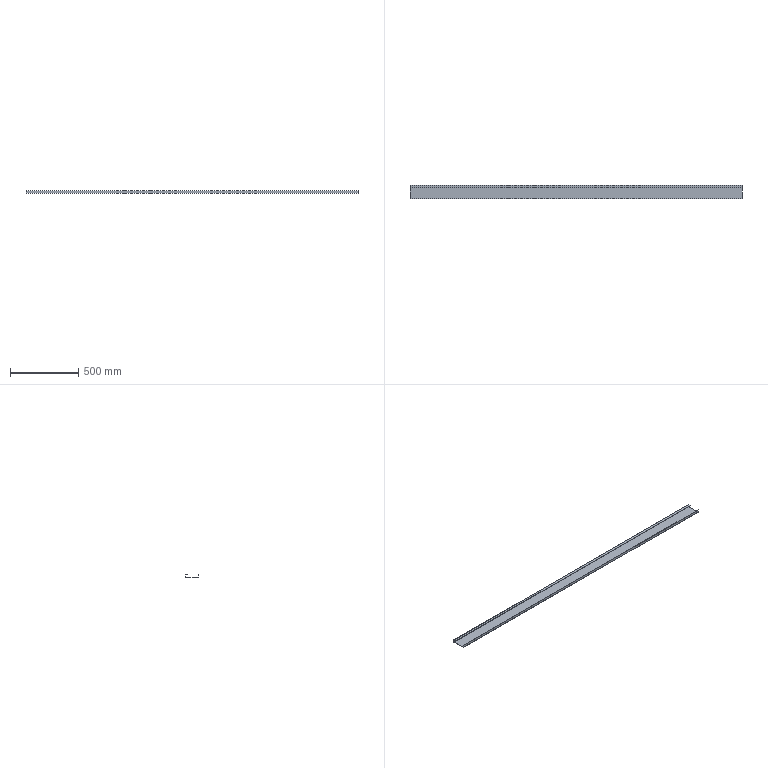Part | STEP file | Powder bin toe plate 4 | 1 solid | 18 faces | box 2430 x 100 x 20 mm | volume 558584 mm3 | plane 12 | cylinder 6 | commonest cylinder face diameters 2 x3 5 x3
STEP:
#1=CARTESIAN_POINT('',(0.,0.,0.));
#2=DIRECTION('',(0.,0.,1.));
#3=DIRECTION('',(1.,0.,0.));
#4=AXIS2_PLACEMENT_3D('',#1,#2,#3);
#5=CARTESIAN_POINT('',(-1215.,1.5,2.5));
#6=VERTEX_POINT('',#5);
#7=CARTESIAN_POINT('',(-1215.,1.5,20.));
#8=VERTEX_POINT('',#7);
#9=CARTESIAN_POINT('',(-1215.,1.5,2.5));
#10=DIRECTION('',(0.,0.,1.));
#11=VECTOR('',#10,1.);
#12=LINE('',#9,#11);
#13=CARTESIAN_POINT('',(1215.,1.5,2.5));
#14=DIRECTION('',(0.,-1.,0.));
#15=DIRECTION('',(0.,0.,-1.));
#16=AXIS2_PLACEMENT_3D('',#13,#14,#15);
#17=PLANE('',#16);
#18=CARTESIAN_POINT('',(0.,-2430.));
#19=DIRECTION('',(-1.,0.));
#20=VECTOR('',#19,1.);
#21=LINE('',#18,#20);
#22=(GEOMETRIC_REPRESENTATION_CONTEXT(2)PARAMETRIC_REPRESENTATION_CONTEXT()REPRESENTATION_CONTEXT('',''));
#23=DEFINITIONAL_REPRESENTATION('',(#21),#22);
#24=PCURVE('',#17,#23);
#25=CARTESIAN_POINT('',(-1215.,2.5,2.5));
#26=DIRECTION('',(-1.,0.,0.));
#27=DIRECTION('',(0.,0.,1.));
#28=AXIS2_PLACEMENT_3D('',#25,#26,#27);
#29=PLANE('',#28);
#30=CARTESIAN_POINT('',(0.,-1.));
#31=DIRECTION('',(1.,0.));
#32=VECTOR('',#31,1.);
#33=LINE('',#30,#32);
#34=(GEOMETRIC_REPRESENTATION_CONTEXT(2)PARAMETRIC_REPRESENTATION_CONTEXT()REPRESENTATION_CONTEXT('',''));
#35=DEFINITIONAL_REPRESENTATION('',(#33),#34);
#36=PCURVE('',#29,#35);
#37=SURFACE_CURVE('',#12,(#24,#36),.PCURVE_S1.);
#38=EDGE_CURVE('',#6,#8,#37,.T.);
#39=ORIENTED_EDGE('',*,*,#38,.T.);
#40=CARTESIAN_POINT('',(1215.,1.5,20.));
#41=VERTEX_POINT('',#40);
#42=CARTESIAN_POINT('',(1215.,1.5,20.));
#43=DIRECTION('',(-1.,0.,0.));
#44=VECTOR('',#43,1.);
#45=LINE('',#42,#44);
#46=CARTESIAN_POINT('',(-17.5,0.));
#47=DIRECTION('',(0.,-1.));
#48=VECTOR('',#47,1.);
#49=LINE('',#46,#48);
#50=(GEOMETRIC_REPRESENTATION_CONTEXT(2)PARAMETRIC_REPRESENTATION_CONTEXT()REPRESENTATION_CONTEXT('',''));
#51=DEFINITIONAL_REPRESENTATION('',(#49),#50);
#52=PCURVE('',#17,#51);
#53=CARTESIAN_POINT('',(1215.,0.,20.));
#54=DIRECTION('',(0.,0.,1.));
#55=DIRECTION('',(1.,0.,0.));
#56=AXIS2_PLACEMENT_3D('',#53,#54,#55);
#57=PLANE('',#56);
#58=CARTESIAN_POINT('',(0.,1.5));
#59=DIRECTION('',(-1.,0.));
#60=VECTOR('',#59,1.);
#61=LINE('',#58,#60);
#62=(GEOMETRIC_REPRESENTATION_CONTEXT(2)PARAMETRIC_REPRESENTATION_CONTEXT()REPRESENTATION_CONTEXT('',''));
#63=DEFINITIONAL_REPRESENTATION('',(#61),#62);
#64=PCURVE('',#57,#63);
#65=SURFACE_CURVE('',#45,(#52,#64),.PCURVE_S1.);
#66=EDGE_CURVE('',#41,#8,#65,.T.);
#67=ORIENTED_EDGE('',*,*,#66,.F.);
#68=CARTESIAN_POINT('',(1215.,1.5,2.5));
#69=VERTEX_POINT('',#68);
#70=CARTESIAN_POINT('',(1215.,1.5,2.5));
#71=DIRECTION('',(0.,0.,1.));
#72=VECTOR('',#71,1.);
#73=LINE('',#70,#72);
#74=CARTESIAN_POINT('',(0.,0.));
#75=DIRECTION('',(-1.,0.));
#76=VECTOR('',#75,1.);
#77=LINE('',#74,#76);
#78=(GEOMETRIC_REPRESENTATION_CONTEXT(2)PARAMETRIC_REPRESENTATION_CONTEXT()REPRESENTATION_CONTEXT('',''));
#79=DEFINITIONAL_REPRESENTATION('',(#77),#78);
#80=PCURVE('',#17,#79);
#81=CARTESIAN_POINT('',(1215.,2.5,2.5));
#82=DIRECTION('',(-1.,0.,0.));
#83=DIRECTION('',(0.,0.,1.));
#84=AXIS2_PLACEMENT_3D('',#81,#82,#83);
#85=PLANE('',#84);
#86=CARTESIAN_POINT('',(0.,-1.));
#87=DIRECTION('',(1.,0.));
#88=VECTOR('',#87,1.);
#89=LINE('',#86,#88);
#90=(GEOMETRIC_REPRESENTATION_CONTEXT(2)PARAMETRIC_REPRESENTATION_CONTEXT()REPRESENTATION_CONTEXT('',''));
#91=DEFINITIONAL_REPRESENTATION('',(#89),#90);
#92=PCURVE('',#85,#91);
#93=SURFACE_CURVE('',#73,(#80,#92),.PCURVE_S1.);
#94=EDGE_CURVE('',#69,#41,#93,.T.);
#95=ORIENTED_EDGE('',*,*,#94,.F.);
#96=CARTESIAN_POINT('',(1215.,1.5,2.5));
#97=DIRECTION('',(-1.,0.,0.));
#98=VECTOR('',#97,1.);
#99=LINE('',#96,#98);
#100=CARTESIAN_POINT('',(0.,0.));
#101=DIRECTION('',(0.,-1.));
#102=VECTOR('',#101,1.);
#103=LINE('',#100,#102);
#104=(GEOMETRIC_REPRESENTATION_CONTEXT(2)PARAMETRIC_REPRESENTATION_CONTEXT()REPRESENTATION_CONTEXT('',''));
#105=DEFINITIONAL_REPRESENTATION('',(#103),#104);
#106=PCURVE('',#17,#105);
#107=CARTESIAN_POINT('',(1215.,2.5,2.5));
#108=DIRECTION('',(-1.,0.,0.));
#109=DIRECTION('',(0.,0.,1.));
#110=AXIS2_PLACEMENT_3D('',#107,#108,#109);
#111=CYLINDRICAL_SURFACE('',#110,1.);
#112=CARTESIAN_POINT('',(4.712,0.));
#113=DIRECTION('',(0.,1.));
#114=VECTOR('',#113,1.);
#115=LINE('',#112,#114);
#116=(GEOMETRIC_REPRESENTATION_CONTEXT(2)PARAMETRIC_REPRESENTATION_CONTEXT()REPRESENTATION_CONTEXT('',''));
#117=DEFINITIONAL_REPRESENTATION('',(#115),#116);
#118=PCURVE('',#111,#117);
#119=SURFACE_CURVE('',#99,(#106,#118),.PCURVE_S1.);
#120=EDGE_CURVE('',#69,#6,#119,.T.);
#121=ORIENTED_EDGE('',*,*,#120,.T.);
#122=EDGE_LOOP('',(#39,#67,#95,#121));
#123=FACE_BOUND('',#122,.T.);
#124=ADVANCED_FACE('',(#123),#17,.F.);
#125=CARTESIAN_POINT('',(-1215.,0.,20.));
#126=VERTEX_POINT('',#125);
#127=CARTESIAN_POINT('',(-1215.,0.,20.));
#128=DIRECTION('',(0.,1.,0.));
#129=VECTOR('',#128,1.);
#130=LINE('',#127,#129);
#131=CARTESIAN_POINT('',(-2430.,0.));
#132=DIRECTION('',(0.,1.));
#133=VECTOR('',#132,1.);
#134=LINE('',#131,#133);
#135=(GEOMETRIC_REPRESENTATION_CONTEXT(2)PARAMETRIC_REPRESENTATION_CONTEXT()REPRESENTATION_CONTEXT('',''));
#136=DEFINITIONAL_REPRESENTATION('',(#134),#135);
#137=PCURVE('',#57,#136);
#138=CARTESIAN_POINT('',(17.5,-2.5));
#139=DIRECTION('',(0.,1.));
#140=VECTOR('',#139,1.);
#141=LINE('',#138,#140);
#142=(GEOMETRIC_REPRESENTATION_CONTEXT(2)PARAMETRIC_REPRESENTATION_CONTEXT()REPRESENTATION_CONTEXT('',''));
#143=DEFINITIONAL_REPRESENTATION('',(#141),#142);
#144=PCURVE('',#29,#143);
#145=SURFACE_CURVE('',#130,(#137,#144),.PCURVE_S1.);
#146=EDGE_CURVE('',#126,#8,#145,.T.);
#147=ORIENTED_EDGE('',*,*,#146,.F.);
#148=CARTESIAN_POINT('',(1215.,0.,20.));
#149=VERTEX_POINT('',#148);
#150=CARTESIAN_POINT('',(1215.,0.,20.));
#151=DIRECTION('',(-1.,0.,0.));
#152=VECTOR('',#151,1.);
#153=LINE('',#150,#152);
#154=CARTESIAN_POINT('',(0.,0.));
#155=DIRECTION('',(-1.,0.));
#156=VECTOR('',#155,1.);
#157=LINE('',#154,#156);
#158=(GEOMETRIC_REPRESENTATION_CONTEXT(2)PARAMETRIC_REPRESENTATION_CONTEXT()REPRESENTATION_CONTEXT('',''));
#159=DEFINITIONAL_REPRESENTATION('',(#157),#158);
#160=PCURVE('',#57,#159);
#161=CARTESIAN_POINT('',(1215.,0.,2.5));
#162=DIRECTION('',(0.,-1.,0.));
#163=DIRECTION('',(0.,0.,-1.));
#164=AXIS2_PLACEMENT_3D('',#161,#162,#163);
#165=PLANE('',#164);
#166=CARTESIAN_POINT('',(-17.5,0.));
#167=DIRECTION('',(0.,-1.));
#168=VECTOR('',#167,1.);
#169=LINE('',#166,#168);
#170=(GEOMETRIC_REPRESENTATION_CONTEXT(2)PARAMETRIC_REPRESENTATION_CONTEXT()REPRESENTATION_CONTEXT('',''));
#171=DEFINITIONAL_REPRESENTATION('',(#169),#170);
#172=PCURVE('',#165,#171);
#173=SURFACE_CURVE('',#153,(#160,#172),.PCURVE_S1.);
#174=EDGE_CURVE('',#149,#126,#173,.T.);
#175=ORIENTED_EDGE('',*,*,#174,.F.);
#176=CARTESIAN_POINT('',(1215.,0.,20.));
#177=DIRECTION('',(0.,1.,0.));
#178=VECTOR('',#177,1.);
#179=LINE('',#176,#178);
#180=CARTESIAN_POINT('',(0.,0.));
#181=DIRECTION('',(0.,1.));
#182=VECTOR('',#181,1.);
#183=LINE('',#180,#182);
#184=(GEOMETRIC_REPRESENTATION_CONTEXT(2)PARAMETRIC_REPRESENTATION_CONTEXT()REPRESENTATION_CONTEXT('',''));
#185=DEFINITIONAL_REPRESENTATION('',(#183),#184);
#186=PCURVE('',#57,#185);
#187=CARTESIAN_POINT('',(17.5,-2.5));
#188=DIRECTION('',(0.,1.));
#189=VECTOR('',#188,1.);
#190=LINE('',#187,#189);
#191=(GEOMETRIC_REPRESENTATION_CONTEXT(2)PARAMETRIC_REPRESENTATION_CONTEXT()REPRESENTATION_CONTEXT('',''));
#192=DEFINITIONAL_REPRESENTATION('',(#190),#191);
#193=PCURVE('',#85,#192);
#194=SURFACE_CURVE('',#179,(#186,#193),.PCURVE_S1.);
#195=EDGE_CURVE('',#149,#41,#194,.T.);
#196=ORIENTED_EDGE('',*,*,#195,.T.);
#197=ORIENTED_EDGE('',*,*,#66,.T.);
#198=EDGE_LOOP('',(#147,#175,#196,#197));
#199=FACE_BOUND('',#198,.T.);
#200=ADVANCED_FACE('',(#199),#57,.T.);
#201=CARTESIAN_POINT('',(-1215.,0.,2.5));
#202=VERTEX_POINT('',#201);
#203=CARTESIAN_POINT('',(-1215.,0.,2.5));
#204=DIRECTION('',(0.,0.,1.));
#205=VECTOR('',#204,1.);
#206=LINE('',#203,#205);
#207=CARTESIAN_POINT('',(0.,-2430.));
#208=DIRECTION('',(-1.,0.));
#209=VECTOR('',#208,1.);
#210=LINE('',#207,#209);
#211=(GEOMETRIC_REPRESENTATION_CONTEXT(2)PARAMETRIC_REPRESENTATION_CONTEXT()REPRESENTATION_CONTEXT('',''));
#212=DEFINITIONAL_REPRESENTATION('',(#210),#211);
#213=PCURVE('',#165,#212);
#214=CARTESIAN_POINT('',(0.,-2.5));
#215=DIRECTION('',(1.,0.));
#216=VECTOR('',#215,1.);
#217=LINE('',#214,#216);
#218=(GEOMETRIC_REPRESENTATION_CONTEXT(2)PARAMETRIC_REPRESENTATION_CONTEXT()REPRESENTATION_CONTEXT('',''));
#219=DEFINITIONAL_REPRESENTATION('',(#217),#218);
#220=PCURVE('',#29,#219);
#221=SURFACE_CURVE('',#206,(#213,#220),.PCURVE_S1.);
#222=EDGE_CURVE('',#202,#126,#221,.T.);
#223=ORIENTED_EDGE('',*,*,#222,.F.);
#224=CARTESIAN_POINT('',(1215.,0.,2.5));
#225=VERTEX_POINT('',#224);
#226=CARTESIAN_POINT('',(1215.,0.,2.5));
#227=DIRECTION('',(-1.,0.,0.));
#228=VECTOR('',#227,1.);
#229=LINE('',#226,#228);
#230=CARTESIAN_POINT('',(0.,0.));
#231=DIRECTION('',(0.,-1.));
#232=VECTOR('',#231,1.);
#233=LINE('',#230,#232);
#234=(GEOMETRIC_REPRESENTATION_CONTEXT(2)PARAMETRIC_REPRESENTATION_CONTEXT()REPRESENTATION_CONTEXT('',''));
#235=DEFINITIONAL_REPRESENTATION('',(#233),#234);
#236=PCURVE('',#165,#235);
#237=CARTESIAN_POINT('',(1215.,2.5,2.5));
#238=DIRECTION('',(-1.,0.,0.));
#239=DIRECTION('',(0.,0.,1.));
#240=AXIS2_PLACEMENT_3D('',#237,#238,#239);
#241=CYLINDRICAL_SURFACE('',#240,2.5);
#242=CARTESIAN_POINT('',(4.712,0.));
#243=DIRECTION('',(0.,1.));
#244=VECTOR('',#243,1.);
#245=LINE('',#242,#244);
#246=(GEOMETRIC_REPRESENTATION_CONTEXT(2)PARAMETRIC_REPRESENTATION_CONTEXT()REPRESENTATION_CONTEXT('',''));
#247=DEFINITIONAL_REPRESENTATION('',(#245),#246);
#248=PCURVE('',#241,#247);
#249=SURFACE_CURVE('',#229,(#236,#248),.PCURVE_S1.);
#250=EDGE_CURVE('',#225,#202,#249,.T.);
#251=ORIENTED_EDGE('',*,*,#250,.F.);
#252=CARTESIAN_POINT('',(1215.,0.,2.5));
#253=DIRECTION('',(0.,0.,1.));
#254=VECTOR('',#253,1.);
#255=LINE('',#252,#254);
#256=CARTESIAN_POINT('',(0.,0.));
#257=DIRECTION('',(-1.,0.));
#258=VECTOR('',#257,1.);
#259=LINE('',#256,#258);
#260=(GEOMETRIC_REPRESENTATION_CONTEXT(2)PARAMETRIC_REPRESENTATION_CONTEXT()REPRESENTATION_CONTEXT('',''));
#261=DEFINITIONAL_REPRESENTATION('',(#259),#260);
#262=PCURVE('',#165,#261);
#263=CARTESIAN_POINT('',(0.,-2.5));
#264=DIRECTION('',(1.,0.));
#265=VECTOR('',#264,1.);
#266=LINE('',#263,#265);
#267=(GEOMETRIC_REPRESENTATION_CONTEXT(2)PARAMETRIC_REPRESENTATION_CONTEXT()REPRESENTATION_CONTEXT('',''));
#268=DEFINITIONAL_REPRESENTATION('',(#266),#267);
#269=PCURVE('',#85,#268);
#270=SURFACE_CURVE('',#255,(#262,#269),.PCURVE_S1.);
#271=EDGE_CURVE('',#225,#149,#270,.T.);
#272=ORIENTED_EDGE('',*,*,#271,.T.);
#273=ORIENTED_EDGE('',*,*,#174,.T.);
#274=EDGE_LOOP('',(#223,#251,#272,#273));
#275=FACE_BOUND('',#274,.T.);
#276=ADVANCED_FACE('',(#275),#165,.T.);
#277=CARTESIAN_POINT('',(-1215.,2.5,0.));
#278=VERTEX_POINT('',#277);
#279=CARTESIAN_POINT('',(-1215.,2.5,2.5));
#280=DIRECTION('',(-1.,0.,0.));
#281=DIRECTION('',(0.,0.,1.));
#282=AXIS2_PLACEMENT_3D('',#279,#280,#281);
#283=CIRCLE('',#282,2.5);
#284=CARTESIAN_POINT('',(0.,2430.));
#285=DIRECTION('',(1.,0.));
#286=VECTOR('',#285,1.);
#287=LINE('',#284,#286);
#288=(GEOMETRIC_REPRESENTATION_CONTEXT(2)PARAMETRIC_REPRESENTATION_CONTEXT()REPRESENTATION_CONTEXT('',''));
#289=DEFINITIONAL_REPRESENTATION('',(#287),#288);
#290=PCURVE('',#241,#289);
#291=CARTESIAN_POINT('',(0.,0.));
#292=DIRECTION('',(1.,0.));
#293=AXIS2_PLACEMENT_2D('',#291,#292);
#294=CIRCLE('',#293,2.5);
#295=(GEOMETRIC_REPRESENTATION_CONTEXT(2)PARAMETRIC_REPRESENTATION_CONTEXT()REPRESENTATION_CONTEXT('',''));
#296=DEFINITIONAL_REPRESENTATION('',(#294),#295);
#297=PCURVE('',#29,#296);
#298=SURFACE_CURVE('',#283,(#290,#297),.PCURVE_S1.);
#299=EDGE_CURVE('',#278,#202,#298,.T.);
#300=ORIENTED_EDGE('',*,*,#299,.F.);
#301=CARTESIAN_POINT('',(1215.,2.5,0.));
#302=VERTEX_POINT('',#301);
#303=CARTESIAN_POINT('',(1215.,2.5,0.));
#304=DIRECTION('',(-1.,0.,0.));
#305=VECTOR('',#304,1.);
#306=LINE('',#303,#305);
#307=CARTESIAN_POINT('',(3.142,0.));
#308=DIRECTION('',(0.,1.));
#309=VECTOR('',#308,1.);
#310=LINE('',#307,#309);
#311=(GEOMETRIC_REPRESENTATION_CONTEXT(2)PARAMETRIC_REPRESENTATION_CONTEXT()REPRESENTATION_CONTEXT('',''));
#312=DEFINITIONAL_REPRESENTATION('',(#310),#311);
#313=PCURVE('',#241,#312);
#314=CARTESIAN_POINT('',(1215.,2.5,0.));
#315=DIRECTION('',(0.,0.,-1.));
#316=DIRECTION('',(-1.,0.,0.));
#317=AXIS2_PLACEMENT_3D('',#314,#315,#316);
#318=PLANE('',#317);
#319=CARTESIAN_POINT('',(0.,0.));
#320=DIRECTION('',(1.,0.));
#321=VECTOR('',#320,1.);
#322=LINE('',#319,#321);
#323=(GEOMETRIC_REPRESENTATION_CONTEXT(2)PARAMETRIC_REPRESENTATION_CONTEXT()REPRESENTATION_CONTEXT('',''));
#324=DEFINITIONAL_REPRESENTATION('',(#322),#323);
#325=PCURVE('',#318,#324);
#326=SURFACE_CURVE('',#306,(#313,#325),.PCURVE_S1.);
#327=EDGE_CURVE('',#302,#278,#326,.T.);
#328=ORIENTED_EDGE('',*,*,#327,.F.);
#329=CARTESIAN_POINT('',(1215.,2.5,2.5));
#330=DIRECTION('',(-1.,0.,0.));
#331=DIRECTION('',(0.,0.,1.));
#332=AXIS2_PLACEMENT_3D('',#329,#330,#331);
#333=CIRCLE('',#332,2.5);
#334=CARTESIAN_POINT('',(0.,0.));
#335=DIRECTION('',(1.,0.));
#336=VECTOR('',#335,1.);
#337=LINE('',#334,#336);
#338=(GEOMETRIC_REPRESENTATION_CONTEXT(2)PARAMETRIC_REPRESENTATION_CONTEXT()REPRESENTATION_CONTEXT('',''));
#339=DEFINITIONAL_REPRESENTATION('',(#337),#338);
#340=PCURVE('',#241,#339);
#341=CARTESIAN_POINT('',(0.,0.));
#342=DIRECTION('',(1.,0.));
#343=AXIS2_PLACEMENT_2D('',#341,#342);
#344=CIRCLE('',#343,2.5);
#345=(GEOMETRIC_REPRESENTATION_CONTEXT(2)PARAMETRIC_REPRESENTATION_CONTEXT()REPRESENTATION_CONTEXT('',''));
#346=DEFINITIONAL_REPRESENTATION('',(#344),#345);
#347=PCURVE('',#85,#346);
#348=SURFACE_CURVE('',#333,(#340,#347),.PCURVE_S1.);
#349=EDGE_CURVE('',#302,#225,#348,.T.);
#350=ORIENTED_EDGE('',*,*,#349,.T.);
#351=ORIENTED_EDGE('',*,*,#250,.T.);
#352=EDGE_LOOP('',(#300,#328,#350,#351));
#353=FACE_BOUND('',#352,.T.);
#354=ADVANCED_FACE('',(#353),#241,.T.);
#355=CARTESIAN_POINT('',(-1215.,97.5,0.));
#356=VERTEX_POINT('',#355);
#357=CARTESIAN_POINT('',(-1215.,2.5,0.));
#358=DIRECTION('',(0.,-1.,0.));
#359=VECTOR('',#358,1.);
#360=LINE('',#357,#359);
#361=CARTESIAN_POINT('',(2430.,0.));
#362=DIRECTION('',(0.,-1.));
#363=VECTOR('',#362,1.);
#364=LINE('',#361,#363);
#365=(GEOMETRIC_REPRESENTATION_CONTEXT(2)PARAMETRIC_REPRESENTATION_CONTEXT()REPRESENTATION_CONTEXT('',''));
#366=DEFINITIONAL_REPRESENTATION('',(#364),#365);
#367=PCURVE('',#318,#366);
#368=CARTESIAN_POINT('',(-2.5,0.));
#369=DIRECTION('',(0.,-1.));
#370=VECTOR('',#369,1.);
#371=LINE('',#368,#370);
#372=(GEOMETRIC_REPRESENTATION_CONTEXT(2)PARAMETRIC_REPRESENTATION_CONTEXT()REPRESENTATION_CONTEXT('',''));
#373=DEFINITIONAL_REPRESENTATION('',(#371),#372);
#374=PCURVE('',#29,#373);
#375=SURFACE_CURVE('',#360,(#367,#374),.PCURVE_S1.);
#376=EDGE_CURVE('',#356,#278,#375,.T.);
#377=ORIENTED_EDGE('',*,*,#376,.F.);
#378=CARTESIAN_POINT('',(1215.,97.5,0.));
#379=VERTEX_POINT('',#378);
#380=CARTESIAN_POINT('',(1215.,97.5,0.));
#381=DIRECTION('',(-1.,0.,0.));
#382=VECTOR('',#381,1.);
#383=LINE('',#380,#382);
#384=CARTESIAN_POINT('',(0.,95.));
#385=DIRECTION('',(1.,0.));
#386=VECTOR('',#385,1.);
#387=LINE('',#384,#386);
#388=(GEOMETRIC_REPRESENTATION_CONTEXT(2)PARAMETRIC_REPRESENTATION_CONTEXT()REPRESENTATION_CONTEXT('',''));
#389=DEFINITIONAL_REPRESENTATION('',(#387),#388);
#390=PCURVE('',#318,#389);
#391=CARTESIAN_POINT('',(1215.,97.5,2.5));
#392=DIRECTION('',(-1.,0.,0.));
#393=DIRECTION('',(0.,0.,1.));
#394=AXIS2_PLACEMENT_3D('',#391,#392,#393);
#395=CYLINDRICAL_SURFACE('',#394,2.5);
#396=CARTESIAN_POINT('',(3.142,0.));
#397=DIRECTION('',(0.,1.));
#398=VECTOR('',#397,1.);
#399=LINE('',#396,#398);
#400=(GEOMETRIC_REPRESENTATION_CONTEXT(2)PARAMETRIC_REPRESENTATION_CONTEXT()REPRESENTATION_CONTEXT('',''));
#401=DEFINITIONAL_REPRESENTATION('',(#399),#400);
#402=PCURVE('',#395,#401);
#403=SURFACE_CURVE('',#383,(#390,#402),.PCURVE_S1.);
#404=EDGE_CURVE('',#379,#356,#403,.T.);
#405=ORIENTED_EDGE('',*,*,#404,.F.);
#406=CARTESIAN_POINT('',(1215.,2.5,0.));
#407=DIRECTION('',(0.,-1.,0.));
#408=VECTOR('',#407,1.);
#409=LINE('',#406,#408);
#410=CARTESIAN_POINT('',(0.,0.));
#411=DIRECTION('',(0.,-1.));
#412=VECTOR('',#411,1.);
#413=LINE('',#410,#412);
#414=(GEOMETRIC_REPRESENTATION_CONTEXT(2)PARAMETRIC_REPRESENTATION_CONTEXT()REPRESENTATION_CONTEXT('',''));
#415=DEFINITIONAL_REPRESENTATION('',(#413),#414);
#416=PCURVE('',#318,#415);
#417=CARTESIAN_POINT('',(-2.5,0.));
#418=DIRECTION('',(0.,-1.));
#419=VECTOR('',#418,1.);
#420=LINE('',#417,#419);
#421=(GEOMETRIC_REPRESENTATION_CONTEXT(2)PARAMETRIC_REPRESENTATION_CONTEXT()REPRESENTATION_CONTEXT('',''));
#422=DEFINITIONAL_REPRESENTATION('',(#420),#421);
#423=PCURVE('',#85,#422);
#424=SURFACE_CURVE('',#409,(#416,#423),.PCURVE_S1.);
#425=EDGE_CURVE('',#379,#302,#424,.T.);
#426=ORIENTED_EDGE('',*,*,#425,.T.);
#427=ORIENTED_EDGE('',*,*,#327,.T.);
#428=EDGE_LOOP('',(#377,#405,#426,#427));
#429=FACE_BOUND('',#428,.T.);
#430=ADVANCED_FACE('',(#429),#318,.T.);
#431=CARTESIAN_POINT('',(-1215.,100.,2.5));
#432=VERTEX_POINT('',#431);
#433=CARTESIAN_POINT('',(-1215.,97.5,2.5));
#434=DIRECTION('',(-1.,0.,0.));
#435=DIRECTION('',(0.,0.,-1.));
#436=AXIS2_PLACEMENT_3D('',#433,#434,#435);
#437=CIRCLE('',#436,2.5);
#438=CARTESIAN_POINT('',(-3.142,2430.));
#439=DIRECTION('',(1.,0.));
#440=VECTOR('',#439,1.);
#441=LINE('',#438,#440);
#442=(GEOMETRIC_REPRESENTATION_CONTEXT(2)PARAMETRIC_REPRESENTATION_CONTEXT()REPRESENTATION_CONTEXT('',''));
#443=DEFINITIONAL_REPRESENTATION('',(#441),#442);
#444=PCURVE('',#395,#443);
#445=CARTESIAN_POINT('',(0.,95.));
#446=DIRECTION('',(-1.,0.));
#447=AXIS2_PLACEMENT_2D('',#445,#446);
#448=CIRCLE('',#447,2.5);
#449=(GEOMETRIC_REPRESENTATION_CONTEXT(2)PARAMETRIC_REPRESENTATION_CONTEXT()REPRESENTATION_CONTEXT('',''));
#450=DEFINITIONAL_REPRESENTATION('',(#448),#449);
#451=PCURVE('',#29,#450);
#452=SURFACE_CURVE('',#437,(#444,#451),.PCURVE_S1.);
#453=EDGE_CURVE('',#432,#356,#452,.T.);
#454=ORIENTED_EDGE('',*,*,#453,.F.);
#455=CARTESIAN_POINT('',(1215.,100.,2.5));
#456=VERTEX_POINT('',#455);
#457=CARTESIAN_POINT('',(1215.,100.,2.5));
#458=DIRECTION('',(-1.,0.,0.));
#459=VECTOR('',#458,1.);
#460=LINE('',#457,#459);
#461=CARTESIAN_POINT('',(1.571,0.));
#462=DIRECTION('',(0.,1.));
#463=VECTOR('',#462,1.);
#464=LINE('',#461,#463);
#465=(GEOMETRIC_REPRESENTATION_CONTEXT(2)PARAMETRIC_REPRESENTATION_CONTEXT()REPRESENTATION_CONTEXT('',''));
#466=DEFINITIONAL_REPRESENTATION('',(#464),#465);
#467=PCURVE('',#395,#466);
#468=CARTESIAN_POINT('',(1215.,100.,2.5));
#469=DIRECTION('',(0.,1.,0.));
#470=DIRECTION('',(0.,0.,1.));
#471=AXIS2_PLACEMENT_3D('',#468,#469,#470);
#472=PLANE('',#471);
#473=CARTESIAN_POINT('',(0.,0.));
#474=DIRECTION('',(0.,-1.));
#475=VECTOR('',#474,1.);
#476=LINE('',#473,#475);
#477=(GEOMETRIC_REPRESENTATION_CONTEXT(2)PARAMETRIC_REPRESENTATION_CONTEXT()REPRESENTATION_CONTEXT('',''));
#478=DEFINITIONAL_REPRESENTATION('',(#476),#477);
#479=PCURVE('',#472,#478);
#480=SURFACE_CURVE('',#460,(#467,#479),.PCURVE_S1.);
#481=EDGE_CURVE('',#456,#432,#480,.T.);
#482=ORIENTED_EDGE('',*,*,#481,.F.);
#483=CARTESIAN_POINT('',(1215.,97.5,2.5));
#484=DIRECTION('',(-1.,0.,0.));
#485=DIRECTION('',(0.,0.,-1.));
#486=AXIS2_PLACEMENT_3D('',#483,#484,#485);
#487=CIRCLE('',#486,2.5);
#488=CARTESIAN_POINT('',(-3.142,0.));
#489=DIRECTION('',(1.,0.));
#490=VECTOR('',#489,1.);
#491=LINE('',#488,#490);
#492=(GEOMETRIC_REPRESENTATION_CONTEXT(2)PARAMETRIC_REPRESENTATION_CONTEXT()REPRESENTATION_CONTEXT('',''));
#493=DEFINITIONAL_REPRESENTATION('',(#491),#492);
#494=PCURVE('',#395,#493);
#495=CARTESIAN_POINT('',(0.,95.));
#496=DIRECTION('',(-1.,0.));
#497=AXIS2_PLACEMENT_2D('',#495,#496);
#498=CIRCLE('',#497,2.5);
#499=(GEOMETRIC_REPRESENTATION_CONTEXT(2)PARAMETRIC_REPRESENTATION_CONTEXT()REPRESENTATION_CONTEXT('',''));
#500=DEFINITIONAL_REPRESENTATION('',(#498),#499);
#501=PCURVE('',#85,#500);
#502=SURFACE_CURVE('',#487,(#494,#501),.PCURVE_S1.);
#503=EDGE_CURVE('',#456,#379,#502,.T.);
#504=ORIENTED_EDGE('',*,*,#503,.T.);
#505=ORIENTED_EDGE('',*,*,#404,.T.);
#506=EDGE_LOOP('',(#454,#482,#504,#505));
#507=FACE_BOUND('',#506,.T.);
#508=ADVANCED_FACE('',(#507),#395,.T.);
#509=CARTESIAN_POINT('',(-1215.,100.,17.5));
#510=VERTEX_POINT('',#509);
#511=CARTESIAN_POINT('',(-1215.,100.,2.5));
#512=DIRECTION('',(0.,0.,-1.));
#513=VECTOR('',#512,1.);
#514=LINE('',#511,#513);
#515=CARTESIAN_POINT('',(0.,-2430.));
#516=DIRECTION('',(-1.,0.));
#517=VECTOR('',#516,1.);
#518=LINE('',#515,#517);
#519=(GEOMETRIC_REPRESENTATION_CONTEXT(2)PARAMETRIC_REPRESENTATION_CONTEXT()REPRESENTATION_CONTEXT('',''));
#520=DEFINITIONAL_REPRESENTATION('',(#518),#519);
#521=PCURVE('',#472,#520);
#522=CARTESIAN_POINT('',(0.,97.5));
#523=DIRECTION('',(-1.,0.));
#524=VECTOR('',#523,1.);
#525=LINE('',#522,#524);
#526=(GEOMETRIC_REPRESENTATION_CONTEXT(2)PARAMETRIC_REPRESENTATION_CONTEXT()REPRESENTATION_CONTEXT('',''));
#527=DEFINITIONAL_REPRESENTATION('',(#525),#526);
#528=PCURVE('',#29,#527);
#529=SURFACE_CURVE('',#514,(#521,#528),.PCURVE_S1.);
#530=EDGE_CURVE('',#510,#432,#529,.T.);
#531=ORIENTED_EDGE('',*,*,#530,.F.);
#532=CARTESIAN_POINT('',(1215.,100.,17.5));
#533=VERTEX_POINT('',#532);
#534=CARTESIAN_POINT('',(1215.,100.,17.5));
#535=DIRECTION('',(-1.,0.,0.));
#536=VECTOR('',#535,1.);
#537=LINE('',#534,#536);
#538=CARTESIAN_POINT('',(15.,0.));
#539=DIRECTION('',(0.,-1.));
#540=VECTOR('',#539,1.);
#541=LINE('',#538,#540);
#542=(GEOMETRIC_REPRESENTATION_CONTEXT(2)PARAMETRIC_REPRESENTATION_CONTEXT()REPRESENTATION_CONTEXT('',''));
#543=DEFINITIONAL_REPRESENTATION('',(#541),#542);
#544=PCURVE('',#472,#543);
#545=CARTESIAN_POINT('',(1215.,97.5,17.5));
#546=DIRECTION('',(-1.,0.,0.));
#547=DIRECTION('',(0.,0.,1.));
#548=AXIS2_PLACEMENT_3D('',#545,#546,#547);
#549=CYLINDRICAL_SURFACE('',#548,2.5);
#550=CARTESIAN_POINT('',(1.571,0.));
#551=DIRECTION('',(0.,1.));
#552=VECTOR('',#551,1.);
#553=LINE('',#550,#552);
#554=(GEOMETRIC_REPRESENTATION_CONTEXT(2)PARAMETRIC_REPRESENTATION_CONTEXT()REPRESENTATION_CONTEXT('',''));
#555=DEFINITIONAL_REPRESENTATION('',(#553),#554);
#556=PCURVE('',#549,#555);
#557=SURFACE_CURVE('',#537,(#544,#556),.PCURVE_S1.);
#558=EDGE_CURVE('',#533,#510,#557,.T.);
#559=ORIENTED_EDGE('',*,*,#558,.F.);
#560=CARTESIAN_POINT('',(1215.,100.,2.5));
#561=DIRECTION('',(0.,0.,-1.));
#562=VECTOR('',#561,1.);
#563=LINE('',#560,#562);
#564=CARTESIAN_POINT('',(0.,0.));
#565=DIRECTION('',(-1.,0.));
#566=VECTOR('',#565,1.);
#567=LINE('',#564,#566);
#568=(GEOMETRIC_REPRESENTATION_CONTEXT(2)PARAMETRIC_REPRESENTATION_CONTEXT()REPRESENTATION_CONTEXT('',''));
#569=DEFINITIONAL_REPRESENTATION('',(#567),#568);
#570=PCURVE('',#472,#569);
#571=CARTESIAN_POINT('',(0.,97.5));
#572=DIRECTION('',(-1.,0.));
#573=VECTOR('',#572,1.);
#574=LINE('',#571,#573);
#575=(GEOMETRIC_REPRESENTATION_CONTEXT(2)PARAMETRIC_REPRESENTATION_CONTEXT()REPRESENTATION_CONTEXT('',''));
#576=DEFINITIONAL_REPRESENTATION('',(#574),#575);
#577=PCURVE('',#85,#576);
#578=SURFACE_CURVE('',#563,(#570,#577),.PCURVE_S1.);
#579=EDGE_CURVE('',#533,#456,#578,.T.);
#580=ORIENTED_EDGE('',*,*,#579,.T.);
#581=ORIENTED_EDGE('',*,*,#481,.T.);
#582=EDGE_LOOP('',(#531,#559,#580,#581));
#583=FACE_BOUND('',#582,.T.);
#584=ADVANCED_FACE('',(#583),#472,.T.);
#585=CARTESIAN_POINT('',(-1215.,97.5,20.));
#586=VERTEX_POINT('',#585);
#587=CARTESIAN_POINT('',(-1215.,97.5,17.5));
#588=DIRECTION('',(-1.,0.,0.));
#589=DIRECTION('',(0.,0.,-1.));
#590=AXIS2_PLACEMENT_3D('',#587,#588,#589);
#591=CIRCLE('',#590,2.5);
#592=CARTESIAN_POINT('',(-3.142,2430.));
#593=DIRECTION('',(1.,0.));
#594=VECTOR('',#593,1.);
#595=LINE('',#592,#594);
#596=(GEOMETRIC_REPRESENTATION_CONTEXT(2)PARAMETRIC_REPRESENTATION_CONTEXT()REPRESENTATION_CONTEXT('',''));
#597=DEFINITIONAL_REPRESENTATION('',(#595),#596);
#598=PCURVE('',#549,#597);
#599=CARTESIAN_POINT('',(15.,95.));
#600=DIRECTION('',(-1.,0.));
#601=AXIS2_PLACEMENT_2D('',#599,#600);
#602=CIRCLE('',#601,2.5);
#603=(GEOMETRIC_REPRESENTATION_CONTEXT(2)PARAMETRIC_REPRESENTATION_CONTEXT()REPRESENTATION_CONTEXT('',''));
#604=DEFINITIONAL_REPRESENTATION('',(#602),#603);
#605=PCURVE('',#29,#604);
#606=SURFACE_CURVE('',#591,(#598,#605),.PCURVE_S1.);
#607=EDGE_CURVE('',#586,#510,#606,.T.);
#608=ORIENTED_EDGE('',*,*,#607,.F.);
#609=CARTESIAN_POINT('',(1215.,97.5,20.));
#610=VERTEX_POINT('',#609);
#611=CARTESIAN_POINT('',(1215.,97.5,20.));
#612=DIRECTION('',(-1.,0.,0.));
#613=VECTOR('',#612,1.);
#614=LINE('',#611,#613);
#615=CARTESIAN_POINT('',(0.,0.));
#616=DIRECTION('',(0.,1.));
#617=VECTOR('',#616,1.);
#618=LINE('',#615,#617);
#619=(GEOMETRIC_REPRESENTATION_CONTEXT(2)PARAMETRIC_REPRESENTATION_CONTEXT()REPRESENTATION_CONTEXT('',''));
#620=DEFINITIONAL_REPRESENTATION('',(#618),#619);
#621=PCURVE('',#549,#620);
#622=CARTESIAN_POINT('',(1215.,97.5,20.));
#623=DIRECTION('',(0.,0.,1.));
#624=DIRECTION('',(1.,0.,0.));
#625=AXIS2_PLACEMENT_3D('',#622,#623,#624);
#626=PLANE('',#625);
#627=CARTESIAN_POINT('',(0.,0.));
#628=DIRECTION('',(-1.,0.));
#629=VECTOR('',#628,1.);
#630=LINE('',#627,#629);
#631=(GEOMETRIC_REPRESENTATION_CONTEXT(2)PARAMETRIC_REPRESENTATION_CONTEXT()REPRESENTATION_CONTEXT('',''));
#632=DEFINITIONAL_REPRESENTATION('',(#630),#631);
#633=PCURVE('',#626,#632);
#634=SURFACE_CURVE('',#614,(#621,#633),.PCURVE_S1.);
#635=EDGE_CURVE('',#610,#586,#634,.T.);
#636=ORIENTED_EDGE('',*,*,#635,.F.);
#637=CARTESIAN_POINT('',(1215.,97.5,17.5));
#638=DIRECTION('',(-1.,0.,0.));
#639=DIRECTION('',(0.,0.,-1.));
#640=AXIS2_PLACEMENT_3D('',#637,#638,#639);
#641=CIRCLE('',#640,2.5);
#642=CARTESIAN_POINT('',(-3.142,0.));
#643=DIRECTION('',(1.,0.));
#644=VECTOR('',#643,1.);
#645=LINE('',#642,#644);
#646=(GEOMETRIC_REPRESENTATION_CONTEXT(2)PARAMETRIC_REPRESENTATION_CONTEXT()REPRESENTATION_CONTEXT('',''));
#647=DEFINITIONAL_REPRESENTATION('',(#645),#646);
#648=PCURVE('',#549,#647);
#649=CARTESIAN_POINT('',(15.,95.));
#650=DIRECTION('',(-1.,0.));
#651=AXIS2_PLACEMENT_2D('',#649,#650);
#652=CIRCLE('',#651,2.5);
#653=(GEOMETRIC_REPRESENTATION_CONTEXT(2)PARAMETRIC_REPRESENTATION_CONTEXT()REPRESENTATION_CONTEXT('',''));
#654=DEFINITIONAL_REPRESENTATION('',(#652),#653);
#655=PCURVE('',#85,#654);
#656=SURFACE_CURVE('',#641,(#648,#655),.PCURVE_S1.);
#657=EDGE_CURVE('',#610,#533,#656,.T.);
#658=ORIENTED_EDGE('',*,*,#657,.T.);
#659=ORIENTED_EDGE('',*,*,#558,.T.);
#660=EDGE_LOOP('',(#608,#636,#658,#659));
#661=FACE_BOUND('',#660,.T.);
#662=ADVANCED_FACE('',(#661),#549,.T.);
#663=CARTESIAN_POINT('',(-1215.,80.,20.));
#664=VERTEX_POINT('',#663);
#665=CARTESIAN_POINT('',(-1215.,97.5,20.));
#666=DIRECTION('',(0.,1.,0.));
#667=VECTOR('',#666,1.);
#668=LINE('',#665,#667);
#669=CARTESIAN_POINT('',(-2430.,0.));
#670=DIRECTION('',(0.,1.));
#671=VECTOR('',#670,1.);
#672=LINE('',#669,#671);
#673=(GEOMETRIC_REPRESENTATION_CONTEXT(2)PARAMETRIC_REPRESENTATION_CONTEXT()REPRESENTATION_CONTEXT('',''));
#674=DEFINITIONAL_REPRESENTATION('',(#672),#673);
#675=PCURVE('',#626,#674);
#676=CARTESIAN_POINT('',(17.5,95.));
#677=DIRECTION('',(0.,1.));
#678=VECTOR('',#677,1.);
#679=LINE('',#676,#678);
#680=(GEOMETRIC_REPRESENTATION_CONTEXT(2)PARAMETRIC_REPRESENTATION_CONTEXT()REPRESENTATION_CONTEXT('',''));
#681=DEFINITIONAL_REPRESENTATION('',(#679),#680);
#682=PCURVE('',#29,#681);
#683=SURFACE_CURVE('',#668,(#675,#682),.PCURVE_S1.);
#684=EDGE_CURVE('',#664,#586,#683,.T.);
#685=ORIENTED_EDGE('',*,*,#684,.F.);
#686=CARTESIAN_POINT('',(1215.,80.,20.));
#687=VERTEX_POINT('',#686);
#688=CARTESIAN_POINT('',(1215.,80.,20.));
#689=DIRECTION('',(-1.,0.,0.));
#690=VECTOR('',#689,1.);
#691=LINE('',#688,#690);
#692=CARTESIAN_POINT('',(0.,-17.5));
#693=DIRECTION('',(-1.,0.));
#694=VECTOR('',#693,1.);
#695=LINE('',#692,#694);
#696=(GEOMETRIC_REPRESENTATION_CONTEXT(2)PARAMETRIC_REPRESENTATION_CONTEXT()REPRESENTATION_CONTEXT('',''));
#697=DEFINITIONAL_REPRESENTATION('',(#695),#696);
#698=PCURVE('',#626,#697);
#699=CARTESIAN_POINT('',(1215.,80.,18.5));
#700=DIRECTION('',(0.,-1.,0.));
#701=DIRECTION('',(0.,0.,-1.));
#702=AXIS2_PLACEMENT_3D('',#699,#700,#701);
#703=PLANE('',#702);
#704=CARTESIAN_POINT('',(-1.5,0.));
#705=DIRECTION('',(0.,-1.));
#706=VECTOR('',#705,1.);
#707=LINE('',#704,#706);
#708=(GEOMETRIC_REPRESENTATION_CONTEXT(2)PARAMETRIC_REPRESENTATION_CONTEXT()REPRESENTATION_CONTEXT('',''));
#709=DEFINITIONAL_REPRESENTATION('',(#707),#708);
#710=PCURVE('',#703,#709);
#711=SURFACE_CURVE('',#691,(#698,#710),.PCURVE_S1.);
#712=EDGE_CURVE('',#687,#664,#711,.T.);
#713=ORIENTED_EDGE('',*,*,#712,.F.);
#714=CARTESIAN_POINT('',(1215.,97.5,20.));
#715=DIRECTION('',(0.,1.,0.));
#716=VECTOR('',#715,1.);
#717=LINE('',#714,#716);
#718=CARTESIAN_POINT('',(0.,0.));
#719=DIRECTION('',(0.,1.));
#720=VECTOR('',#719,1.);
#721=LINE('',#718,#720);
#722=(GEOMETRIC_REPRESENTATION_CONTEXT(2)PARAMETRIC_REPRESENTATION_CONTEXT()REPRESENTATION_CONTEXT('',''));
#723=DEFINITIONAL_REPRESENTATION('',(#721),#722);
#724=PCURVE('',#626,#723);
#725=CARTESIAN_POINT('',(17.5,95.));
#726=DIRECTION('',(0.,1.));
#727=VECTOR('',#726,1.);
#728=LINE('',#725,#727);
#729=(GEOMETRIC_REPRESENTATION_CONTEXT(2)PARAMETRIC_REPRESENTATION_CONTEXT()REPRESENTATION_CONTEXT('',''));
#730=DEFINITIONAL_REPRESENTATION('',(#728),#729);
#731=PCURVE('',#85,#730);
#732=SURFACE_CURVE('',#717,(#724,#731),.PCURVE_S1.);
#733=EDGE_CURVE('',#687,#610,#732,.T.);
#734=ORIENTED_EDGE('',*,*,#733,.T.);
#735=ORIENTED_EDGE('',*,*,#635,.T.);
#736=EDGE_LOOP('',(#685,#713,#734,#735));
#737=FACE_BOUND('',#736,.T.);
#738=ADVANCED_FACE('',(#737),#626,.T.);
#739=CARTESIAN_POINT('',(-1215.,80.,18.5));
#740=VERTEX_POINT('',#739);
#741=CARTESIAN_POINT('',(-1215.,80.,18.5));
#742=DIRECTION('',(0.,0.,1.));
#743=VECTOR('',#742,1.);
#744=LINE('',#741,#743);
#745=CARTESIAN_POINT('',(0.,-2430.));
#746=DIRECTION('',(-1.,0.));
#747=VECTOR('',#746,1.);
#748=LINE('',#745,#747);
#749=(GEOMETRIC_REPRESENTATION_CONTEXT(2)PARAMETRIC_REPRESENTATION_CONTEXT()REPRESENTATION_CONTEXT('',''));
#750=DEFINITIONAL_REPRESENTATION('',(#748),#749);
#751=PCURVE('',#703,#750);
#752=CARTESIAN_POINT('',(16.,77.5));
#753=DIRECTION('',(1.,0.));
#754=VECTOR('',#753,1.);
#755=LINE('',#752,#754);
#756=(GEOMETRIC_REPRESENTATION_CONTEXT(2)PARAMETRIC_REPRESENTATION_CONTEXT()REPRESENTATION_CONTEXT('',''));
#757=DEFINITIONAL_REPRESENTATION('',(#755),#756);
#758=PCURVE('',#29,#757);
#759=SURFACE_CURVE('',#744,(#751,#758),.PCURVE_S1.);
#760=EDGE_CURVE('',#740,#664,#759,.T.);
#761=ORIENTED_EDGE('',*,*,#760,.F.);
#762=CARTESIAN_POINT('',(1215.,80.,18.5));
#763=VERTEX_POINT('',#762);
#764=CARTESIAN_POINT('',(1215.,80.,18.5));
#765=DIRECTION('',(-1.,0.,0.));
#766=VECTOR('',#765,1.);
#767=LINE('',#764,#766);
#768=CARTESIAN_POINT('',(0.,0.));
#769=DIRECTION('',(0.,-1.));
#770=VECTOR('',#769,1.);
#771=LINE('',#768,#770);
#772=(GEOMETRIC_REPRESENTATION_CONTEXT(2)PARAMETRIC_REPRESENTATION_CONTEXT()REPRESENTATION_CONTEXT('',''));
#773=DEFINITIONAL_REPRESENTATION('',(#771),#772);
#774=PCURVE('',#703,#773);
#775=CARTESIAN_POINT('',(1215.,97.5,18.5));
#776=DIRECTION('',(0.,0.,1.));
#777=DIRECTION('',(1.,0.,0.));
#778=AXIS2_PLACEMENT_3D('',#775,#776,#777);
#779=PLANE('',#778);
#780=CARTESIAN_POINT('',(0.,-17.5));
#781=DIRECTION('',(-1.,0.));
#782=VECTOR('',#781,1.);
#783=LINE('',#780,#782);
#784=(GEOMETRIC_REPRESENTATION_CONTEXT(2)PARAMETRIC_REPRESENTATION_CONTEXT()REPRESENTATION_CONTEXT('',''));
#785=DEFINITIONAL_REPRESENTATION('',(#783),#784);
#786=PCURVE('',#779,#785);
#787=SURFACE_CURVE('',#767,(#774,#786),.PCURVE_S1.);
#788=EDGE_CURVE('',#763,#740,#787,.T.);
#789=ORIENTED_EDGE('',*,*,#788,.F.);
#790=CARTESIAN_POINT('',(1215.,80.,18.5));
#791=DIRECTION('',(0.,0.,1.));
#792=VECTOR('',#791,1.);
#793=LINE('',#790,#792);
#794=CARTESIAN_POINT('',(0.,0.));
#795=DIRECTION('',(-1.,0.));
#796=VECTOR('',#795,1.);
#797=LINE('',#794,#796);
#798=(GEOMETRIC_REPRESENTATION_CONTEXT(2)PARAMETRIC_REPRESENTATION_CONTEXT()REPRESENTATION_CONTEXT('',''));
#799=DEFINITIONAL_REPRESENTATION('',(#797),#798);
#800=PCURVE('',#703,#799);
#801=CARTESIAN_POINT('',(16.,77.5));
#802=DIRECTION('',(1.,0.));
#803=VECTOR('',#802,1.);
#804=LINE('',#801,#803);
#805=(GEOMETRIC_REPRESENTATION_CONTEXT(2)PARAMETRIC_REPRESENTATION_CONTEXT()REPRESENTATION_CONTEXT('',''));
#806=DEFINITIONAL_REPRESENTATION('',(#804),#805);
#807=PCURVE('',#85,#806);
#808=SURFACE_CURVE('',#793,(#800,#807),.PCURVE_S1.);
#809=EDGE_CURVE('',#763,#687,#808,.T.);
#810=ORIENTED_EDGE('',*,*,#809,.T.);
#811=ORIENTED_EDGE('',*,*,#712,.T.);
#812=EDGE_LOOP('',(#761,#789,#810,#811));
#813=FACE_BOUND('',#812,.T.);
#814=ADVANCED_FACE('',(#813),#703,.T.);
#815=CARTESIAN_POINT('',(-1215.,97.5,18.5));
#816=VERTEX_POINT('',#815);
#817=CARTESIAN_POINT('',(-1215.,97.5,18.5));
#818=DIRECTION('',(0.,1.,0.));
#819=VECTOR('',#818,1.);
#820=LINE('',#817,#819);
#821=CARTESIAN_POINT('',(-2430.,0.));
#822=DIRECTION('',(0.,1.));
#823=VECTOR('',#822,1.);
#824=LINE('',#821,#823);
#825=(GEOMETRIC_REPRESENTATION_CONTEXT(2)PARAMETRIC_REPRESENTATION_CONTEXT()REPRESENTATION_CONTEXT('',''));
#826=DEFINITIONAL_REPRESENTATION('',(#824),#825);
#827=PCURVE('',#779,#826);
#828=CARTESIAN_POINT('',(16.,95.));
#829=DIRECTION('',(0.,1.));
#830=VECTOR('',#829,1.);
#831=LINE('',#828,#830);
#832=(GEOMETRIC_REPRESENTATION_CONTEXT(2)PARAMETRIC_REPRESENTATION_CONTEXT()REPRESENTATION_CONTEXT('',''));
#833=DEFINITIONAL_REPRESENTATION('',(#831),#832);
#834=PCURVE('',#29,#833);
#835=SURFACE_CURVE('',#820,(#827,#834),.PCURVE_S1.);
#836=EDGE_CURVE('',#740,#816,#835,.T.);
#837=ORIENTED_EDGE('',*,*,#836,.T.);
#838=CARTESIAN_POINT('',(1215.,97.5,18.5));
#839=VERTEX_POINT('',#838);
#840=CARTESIAN_POINT('',(1215.,97.5,18.5));
#841=DIRECTION('',(-1.,0.,0.));
#842=VECTOR('',#841,1.);
#843=LINE('',#840,#842);
#844=CARTESIAN_POINT('',(0.,0.));
#845=DIRECTION('',(-1.,0.));
#846=VECTOR('',#845,1.);
#847=LINE('',#844,#846);
#848=(GEOMETRIC_REPRESENTATION_CONTEXT(2)PARAMETRIC_REPRESENTATION_CONTEXT()REPRESENTATION_CONTEXT('',''));
#849=DEFINITIONAL_REPRESENTATION('',(#847),#848);
#850=PCURVE('',#779,#849);
#851=CARTESIAN_POINT('',(1215.,97.5,17.5));
#852=DIRECTION('',(-1.,0.,0.));
#853=DIRECTION('',(0.,0.,1.));
#854=AXIS2_PLACEMENT_3D('',#851,#852,#853);
#855=CYLINDRICAL_SURFACE('',#854,1.);
#856=CARTESIAN_POINT('',(0.,0.));
#857=DIRECTION('',(0.,1.));
#858=VECTOR('',#857,1.);
#859=LINE('',#856,#858);
#860=(GEOMETRIC_REPRESENTATION_CONTEXT(2)PARAMETRIC_REPRESENTATION_CONTEXT()REPRESENTATION_CONTEXT('',''));
#861=DEFINITIONAL_REPRESENTATION('',(#859),#860);
#862=PCURVE('',#855,#861);
#863=SURFACE_CURVE('',#843,(#850,#862),.PCURVE_S1.);
#864=EDGE_CURVE('',#839,#816,#863,.T.);
#865=ORIENTED_EDGE('',*,*,#864,.F.);
#866=CARTESIAN_POINT('',(1215.,97.5,18.5));
#867=DIRECTION('',(0.,1.,0.));
#868=VECTOR('',#867,1.);
#869=LINE('',#866,#868);
#870=CARTESIAN_POINT('',(0.,0.));
#871=DIRECTION('',(0.,1.));
#872=VECTOR('',#871,1.);
#873=LINE('',#870,#872);
#874=(GEOMETRIC_REPRESENTATION_CONTEXT(2)PARAMETRIC_REPRESENTATION_CONTEXT()REPRESENTATION_CONTEXT('',''));
#875=DEFINITIONAL_REPRESENTATION('',(#873),#874);
#876=PCURVE('',#779,#875);
#877=CARTESIAN_POINT('',(16.,95.));
#878=DIRECTION('',(0.,1.));
#879=VECTOR('',#878,1.);
#880=LINE('',#877,#879);
#881=(GEOMETRIC_REPRESENTATION_CONTEXT(2)PARAMETRIC_REPRESENTATION_CONTEXT()REPRESENTATION_CONTEXT('',''));
#882=DEFINITIONAL_REPRESENTATION('',(#880),#881);
#883=PCURVE('',#85,#882);
#884=SURFACE_CURVE('',#869,(#876,#883),.PCURVE_S1.);
#885=EDGE_CURVE('',#763,#839,#884,.T.);
#886=ORIENTED_EDGE('',*,*,#885,.F.);
#887=ORIENTED_EDGE('',*,*,#788,.T.);
#888=EDGE_LOOP('',(#837,#865,#886,#887));
#889=FACE_BOUND('',#888,.T.);
#890=ADVANCED_FACE('',(#889),#779,.F.);
#891=ORIENTED_EDGE('',*,*,#864,.F.);
#892=CARTESIAN_POINT('',(1215.,98.5,17.5));
#893=VERTEX_POINT('',#892);
#894=CARTESIAN_POINT('',(1215.,97.5,17.5));
#895=DIRECTION('',(-1.,0.,0.));
#896=DIRECTION('',(0.,0.,-1.));
#897=AXIS2_PLACEMENT_3D('',#894,#895,#896);
#898=CIRCLE('',#897,1.);
#899=CARTESIAN_POINT('',(-3.142,0.));
#900=DIRECTION('',(1.,0.));
#901=VECTOR('',#900,1.);
#902=LINE('',#899,#901);
#903=(GEOMETRIC_REPRESENTATION_CONTEXT(2)PARAMETRIC_REPRESENTATION_CONTEXT()REPRESENTATION_CONTEXT('',''));
#904=DEFINITIONAL_REPRESENTATION('',(#902),#903);
#905=PCURVE('',#855,#904);
#906=CARTESIAN_POINT('',(15.,95.));
#907=DIRECTION('',(-1.,0.));
#908=AXIS2_PLACEMENT_2D('',#906,#907);
#909=CIRCLE('',#908,1.);
#910=(GEOMETRIC_REPRESENTATION_CONTEXT(2)PARAMETRIC_REPRESENTATION_CONTEXT()REPRESENTATION_CONTEXT('',''));
#911=DEFINITIONAL_REPRESENTATION('',(#909),#910);
#912=PCURVE('',#85,#911);
#913=SURFACE_CURVE('',#898,(#905,#912),.PCURVE_S1.);
#914=EDGE_CURVE('',#839,#893,#913,.T.);
#915=ORIENTED_EDGE('',*,*,#914,.T.);
#916=CARTESIAN_POINT('',(-1215.,98.5,17.5));
#917=VERTEX_POINT('',#916);
#918=CARTESIAN_POINT('',(1215.,98.5,17.5));
#919=DIRECTION('',(-1.,0.,0.));
#920=VECTOR('',#919,1.);
#921=LINE('',#918,#920);
#922=CARTESIAN_POINT('',(1.571,0.));
#923=DIRECTION('',(0.,1.));
#924=VECTOR('',#923,1.);
#925=LINE('',#922,#924);
#926=(GEOMETRIC_REPRESENTATION_CONTEXT(2)PARAMETRIC_REPRESENTATION_CONTEXT()REPRESENTATION_CONTEXT('',''));
#927=DEFINITIONAL_REPRESENTATION('',(#925),#926);
#928=PCURVE('',#855,#927);
#929=CARTESIAN_POINT('',(1215.,98.5,2.5));
#930=DIRECTION('',(0.,1.,0.));
#931=DIRECTION('',(0.,0.,1.));
#932=AXIS2_PLACEMENT_3D('',#929,#930,#931);
#933=PLANE('',#932);
#934=CARTESIAN_POINT('',(15.,0.));
#935=DIRECTION('',(0.,-1.));
#936=VECTOR('',#935,1.);
#937=LINE('',#934,#936);
#938=(GEOMETRIC_REPRESENTATION_CONTEXT(2)PARAMETRIC_REPRESENTATION_CONTEXT()REPRESENTATION_CONTEXT('',''));
#939=DEFINITIONAL_REPRESENTATION('',(#937),#938);
#940=PCURVE('',#933,#939);
#941=SURFACE_CURVE('',#921,(#928,#940),.PCURVE_S1.);
#942=EDGE_CURVE('',#893,#917,#941,.T.);
#943=ORIENTED_EDGE('',*,*,#942,.T.);
#944=CARTESIAN_POINT('',(-1215.,97.5,17.5));
#945=DIRECTION('',(-1.,0.,0.));
#946=DIRECTION('',(0.,0.,-1.));
#947=AXIS2_PLACEMENT_3D('',#944,#945,#946);
#948=CIRCLE('',#947,1.);
#949=CARTESIAN_POINT('',(-3.142,2430.));
#950=DIRECTION('',(1.,0.));
#951=VECTOR('',#950,1.);
#952=LINE('',#949,#951);
#953=(GEOMETRIC_REPRESENTATION_CONTEXT(2)PARAMETRIC_REPRESENTATION_CONTEXT()REPRESENTATION_CONTEXT('',''));
#954=DEFINITIONAL_REPRESENTATION('',(#952),#953);
#955=PCURVE('',#855,#954);
#956=CARTESIAN_POINT('',(15.,95.));
#957=DIRECTION('',(-1.,0.));
#958=AXIS2_PLACEMENT_2D('',#956,#957);
#959=CIRCLE('',#958,1.);
#960=(GEOMETRIC_REPRESENTATION_CONTEXT(2)PARAMETRIC_REPRESENTATION_CONTEXT()REPRESENTATION_CONTEXT('',''));
#961=DEFINITIONAL_REPRESENTATION('',(#959),#960);
#962=PCURVE('',#29,#961);
#963=SURFACE_CURVE('',#948,(#955,#962),.PCURVE_S1.);
#964=EDGE_CURVE('',#816,#917,#963,.T.);
#965=ORIENTED_EDGE('',*,*,#964,.F.);
#966=EDGE_LOOP('',(#891,#915,#943,#965));
#967=FACE_BOUND('',#966,.F.);
#968=ADVANCED_FACE('',(#967),#855,.F.);
#969=CARTESIAN_POINT('',(-1215.,98.5,2.5));
#970=VERTEX_POINT('',#969);
#971=CARTESIAN_POINT('',(-1215.,98.5,2.5));
#972=DIRECTION('',(0.,0.,-1.));
#973=VECTOR('',#972,1.);
#974=LINE('',#971,#973);
#975=CARTESIAN_POINT('',(0.,-2430.));
#976=DIRECTION('',(-1.,0.));
#977=VECTOR('',#976,1.);
#978=LINE('',#975,#977);
#979=(GEOMETRIC_REPRESENTATION_CONTEXT(2)PARAMETRIC_REPRESENTATION_CONTEXT()REPRESENTATION_CONTEXT('',''));
#980=DEFINITIONAL_REPRESENTATION('',(#978),#979);
#981=PCURVE('',#933,#980);
#982=CARTESIAN_POINT('',(0.,96.));
#983=DIRECTION('',(-1.,0.));
#984=VECTOR('',#983,1.);
#985=LINE('',#982,#984);
#986=(GEOMETRIC_REPRESENTATION_CONTEXT(2)PARAMETRIC_REPRESENTATION_CONTEXT()REPRESENTATION_CONTEXT('',''));
#987=DEFINITIONAL_REPRESENTATION('',(#985),#986);
#988=PCURVE('',#29,#987);
#989=SURFACE_CURVE('',#974,(#981,#988),.PCURVE_S1.);
#990=EDGE_CURVE('',#917,#970,#989,.T.);
#991=ORIENTED_EDGE('',*,*,#990,.T.);
#992=CARTESIAN_POINT('',(1215.,98.5,2.5));
#993=VERTEX_POINT('',#992);
#994=CARTESIAN_POINT('',(1215.,98.5,2.5));
#995=DIRECTION('',(-1.,0.,0.));
#996=VECTOR('',#995,1.);
#997=LINE('',#994,#996);
#998=CARTESIAN_POINT('',(0.,0.));
#999=DIRECTION('',(0.,-1.));
#1000=VECTOR('',#999,1.);
#1001=LINE('',#998,#1000);
#1002=(GEOMETRIC_REPRESENTATION_CONTEXT(2)PARAMETRIC_REPRESENTATION_CONTEXT()REPRESENTATION_CONTEXT('',''));
#1003=DEFINITIONAL_REPRESENTATION('',(#1001),#1002);
#1004=PCURVE('',#933,#1003);
#1005=CARTESIAN_POINT('',(1215.,97.5,2.5));
#1006=DIRECTION('',(-1.,0.,0.));
#1007=DIRECTION('',(0.,0.,1.));
#1008=AXIS2_PLACEMENT_3D('',#1005,#1006,#1007);
#1009=CYLINDRICAL_SURFACE('',#1008,1.);
#1010=CARTESIAN_POINT('',(1.571,0.));
#1011=DIRECTION('',(0.,1.));
#1012=VECTOR('',#1011,1.);
#1013=LINE('',#1010,#1012);
#1014=(GEOMETRIC_REPRESENTATION_CONTEXT(2)PARAMETRIC_REPRESENTATION_CONTEXT()REPRESENTATION_CONTEXT('',''));
#1015=DEFINITIONAL_REPRESENTATION('',(#1013),#1014);
#1016=PCURVE('',#1009,#1015);
#1017=SURFACE_CURVE('',#997,(#1004,#1016),.PCURVE_S1.);
#1018=EDGE_CURVE('',#993,#970,#1017,.T.);
#1019=ORIENTED_EDGE('',*,*,#1018,.F.);
#1020=CARTESIAN_POINT('',(1215.,98.5,2.5));
#1021=DIRECTION('',(0.,0.,-1.));
#1022=VECTOR('',#1021,1.);
#1023=LINE('',#1020,#1022);
#1024=CARTESIAN_POINT('',(0.,0.));
#1025=DIRECTION('',(-1.,0.));
#1026=VECTOR('',#1025,1.);
#1027=LINE('',#1024,#1026);
#1028=(GEOMETRIC_REPRESENTATION_CONTEXT(2)PARAMETRIC_REPRESENTATION_CONTEXT()REPRESENTATION_CONTEXT('',''));
#1029=DEFINITIONAL_REPRESENTATION('',(#1027),#1028);
#1030=PCURVE('',#933,#1029);
#1031=CARTESIAN_POINT('',(0.,96.));
#1032=DIRECTION('',(-1.,0.));
#1033=VECTOR('',#1032,1.);
#1034=LINE('',#1031,#1033);
#1035=(GEOMETRIC_REPRESENTATION_CONTEXT(2)PARAMETRIC_REPRESENTATION_CONTEXT()REPRESENTATION_CONTEXT('',''));
#1036=DEFINITIONAL_REPRESENTATION('',(#1034),#1035);
#1037=PCURVE('',#85,#1036);
#1038=SURFACE_CURVE('',#1023,(#1030,#1037),.PCURVE_S1.);
#1039=EDGE_CURVE('',#893,#993,#1038,.T.);
#1040=ORIENTED_EDGE('',*,*,#1039,.F.);
#1041=ORIENTED_EDGE('',*,*,#942,.T.);
#1042=EDGE_LOOP('',(#991,#1019,#1040,#1041));
#1043=FACE_BOUND('',#1042,.T.);
#1044=ADVANCED_FACE('',(#1043),#933,.F.);
#1045=ORIENTED_EDGE('',*,*,#1018,.F.);
#1046=CARTESIAN_POINT('',(1215.,97.5,1.5));
#1047=VERTEX_POINT('',#1046);
#1048=CARTESIAN_POINT('',(1215.,97.5,2.5));
#1049=DIRECTION('',(-1.,0.,0.));
#1050=DIRECTION('',(0.,0.,-1.));
#1051=AXIS2_PLACEMENT_3D('',#1048,#1049,#1050);
#1052=CIRCLE('',#1051,1.);
#1053=CARTESIAN_POINT('',(-3.142,0.));
#1054=DIRECTION('',(1.,0.));
#1055=VECTOR('',#1054,1.);
#1056=LINE('',#1053,#1055);
#1057=(GEOMETRIC_REPRESENTATION_CONTEXT(2)PARAMETRIC_REPRESENTATION_CONTEXT()REPRESENTATION_CONTEXT('',''));
#1058=DEFINITIONAL_REPRESENTATION('',(#1056),#1057);
#1059=PCURVE('',#1009,#1058);
#1060=CARTESIAN_POINT('',(0.,95.));
#1061=DIRECTION('',(-1.,0.));
#1062=AXIS2_PLACEMENT_2D('',#1060,#1061);
#1063=CIRCLE('',#1062,1.);
#1064=(GEOMETRIC_REPRESENTATION_CONTEXT(2)PARAMETRIC_REPRESENTATION_CONTEXT()REPRESENTATION_CONTEXT('',''));
#1065=DEFINITIONAL_REPRESENTATION('',(#1063),#1064);
#1066=PCURVE('',#85,#1065);
#1067=SURFACE_CURVE('',#1052,(#1059,#1066),.PCURVE_S1.);
#1068=EDGE_CURVE('',#993,#1047,#1067,.T.);
#1069=ORIENTED_EDGE('',*,*,#1068,.T.);
#1070=CARTESIAN_POINT('',(-1215.,97.5,1.5));
#1071=VERTEX_POINT('',#1070);
#1072=CARTESIAN_POINT('',(1215.,97.5,1.5));
#1073=DIRECTION('',(-1.,0.,0.));
#1074=VECTOR('',#1073,1.);
#1075=LINE('',#1072,#1074);
#1076=CARTESIAN_POINT('',(3.142,0.));
#1077=DIRECTION('',(0.,1.));
#1078=VECTOR('',#1077,1.);
#1079=LINE('',#1076,#1078);
#1080=(GEOMETRIC_REPRESENTATION_CONTEXT(2)PARAMETRIC_REPRESENTATION_CONTEXT()REPRESENTATION_CONTEXT('',''));
#1081=DEFINITIONAL_REPRESENTATION('',(#1079),#1080);
#1082=PCURVE('',#1009,#1081);
#1083=CARTESIAN_POINT('',(1215.,2.5,1.5));
#1084=DIRECTION('',(0.,0.,-1.));
#1085=DIRECTION('',(-1.,0.,0.));
#1086=AXIS2_PLACEMENT_3D('',#1083,#1084,#1085);
#1087=PLANE('',#1086);
#1088=CARTESIAN_POINT('',(0.,95.));
#1089=DIRECTION('',(1.,0.));
#1090=VECTOR('',#1089,1.);
#1091=LINE('',#1088,#1090);
#1092=(GEOMETRIC_REPRESENTATION_CONTEXT(2)PARAMETRIC_REPRESENTATION_CONTEXT()REPRESENTATION_CONTEXT('',''));
#1093=DEFINITIONAL_REPRESENTATION('',(#1091),#1092);
#1094=PCURVE('',#1087,#1093);
#1095=SURFACE_CURVE('',#1075,(#1082,#1094),.PCURVE_S1.);
#1096=EDGE_CURVE('',#1047,#1071,#1095,.T.);
#1097=ORIENTED_EDGE('',*,*,#1096,.T.);
#1098=CARTESIAN_POINT('',(-1215.,97.5,2.5));
#1099=DIRECTION('',(-1.,0.,0.));
#1100=DIRECTION('',(0.,0.,-1.));
#1101=AXIS2_PLACEMENT_3D('',#1098,#1099,#1100);
#1102=CIRCLE('',#1101,1.);
#1103=CARTESIAN_POINT('',(-3.142,2430.));
#1104=DIRECTION('',(1.,0.));
#1105=VECTOR('',#1104,1.);
#1106=LINE('',#1103,#1105);
#1107=(GEOMETRIC_REPRESENTATION_CONTEXT(2)PARAMETRIC_REPRESENTATION_CONTEXT()REPRESENTATION_CONTEXT('',''));
#1108=DEFINITIONAL_REPRESENTATION('',(#1106),#1107);
#1109=PCURVE('',#1009,#1108);
#1110=CARTESIAN_POINT('',(0.,95.));
#1111=DIRECTION('',(-1.,0.));
#1112=AXIS2_PLACEMENT_2D('',#1110,#1111);
#1113=CIRCLE('',#1112,1.);
#1114=(GEOMETRIC_REPRESENTATION_CONTEXT(2)PARAMETRIC_REPRESENTATION_CONTEXT()REPRESENTATION_CONTEXT('',''));
#1115=DEFINITIONAL_REPRESENTATION('',(#1113),#1114);
#1116=PCURVE('',#29,#1115);
#1117=SURFACE_CURVE('',#1102,(#1109,#1116),.PCURVE_S1.);
#1118=EDGE_CURVE('',#970,#1071,#1117,.T.);
#1119=ORIENTED_EDGE('',*,*,#1118,.F.);
#1120=EDGE_LOOP('',(#1045,#1069,#1097,#1119));
#1121=FACE_BOUND('',#1120,.F.);
#1122=ADVANCED_FACE('',(#1121),#1009,.F.);
#1123=CARTESIAN_POINT('',(-1215.,2.5,1.5));
#1124=VERTEX_POINT('',#1123);
#1125=CARTESIAN_POINT('',(-1215.,2.5,1.5));
#1126=DIRECTION('',(0.,-1.,0.));
#1127=VECTOR('',#1126,1.);
#1128=LINE('',#1125,#1127);
#1129=CARTESIAN_POINT('',(2430.,0.));
#1130=DIRECTION('',(0.,-1.));
#1131=VECTOR('',#1130,1.);
#1132=LINE('',#1129,#1131);
#1133=(GEOMETRIC_REPRESENTATION_CONTEXT(2)PARAMETRIC_REPRESENTATION_CONTEXT()REPRESENTATION_CONTEXT('',''));
#1134=DEFINITIONAL_REPRESENTATION('',(#1132),#1133);
#1135=PCURVE('',#1087,#1134);
#1136=CARTESIAN_POINT('',(-1.,0.));
#1137=DIRECTION('',(0.,-1.));
#1138=VECTOR('',#1137,1.);
#1139=LINE('',#1136,#1138);
#1140=(GEOMETRIC_REPRESENTATION_CONTEXT(2)PARAMETRIC_REPRESENTATION_CONTEXT()REPRESENTATION_CONTEXT('',''));
#1141=DEFINITIONAL_REPRESENTATION('',(#1139),#1140);
#1142=PCURVE('',#29,#1141);
#1143=SURFACE_CURVE('',#1128,(#1135,#1142),.PCURVE_S1.);
#1144=EDGE_CURVE('',#1071,#1124,#1143,.T.);
#1145=ORIENTED_EDGE('',*,*,#1144,.T.);
#1146=CARTESIAN_POINT('',(1215.,2.5,1.5));
#1147=VERTEX_POINT('',#1146);
#1148=CARTESIAN_POINT('',(1215.,2.5,1.5));
#1149=DIRECTION('',(-1.,0.,0.));
#1150=VECTOR('',#1149,1.);
#1151=LINE('',#1148,#1150);
#1152=CARTESIAN_POINT('',(0.,0.));
#1153=DIRECTION('',(1.,0.));
#1154=VECTOR('',#1153,1.);
#1155=LINE('',#1152,#1154);
#1156=(GEOMETRIC_REPRESENTATION_CONTEXT(2)PARAMETRIC_REPRESENTATION_CONTEXT()REPRESENTATION_CONTEXT('',''));
#1157=DEFINITIONAL_REPRESENTATION('',(#1155),#1156);
#1158=PCURVE('',#1087,#1157);
#1159=CARTESIAN_POINT('',(3.142,0.));
#1160=DIRECTION('',(0.,1.));
#1161=VECTOR('',#1160,1.);
#1162=LINE('',#1159,#1161);
#1163=(GEOMETRIC_REPRESENTATION_CONTEXT(2)PARAMETRIC_REPRESENTATION_CONTEXT()REPRESENTATION_CONTEXT('',''));
#1164=DEFINITIONAL_REPRESENTATION('',(#1162),#1163);
#1165=PCURVE('',#111,#1164);
#1166=SURFACE_CURVE('',#1151,(#1158,#1165),.PCURVE_S1.);
#1167=EDGE_CURVE('',#1147,#1124,#1166,.T.);
#1168=ORIENTED_EDGE('',*,*,#1167,.F.);
#1169=CARTESIAN_POINT('',(1215.,2.5,1.5));
#1170=DIRECTION('',(0.,-1.,0.));
#1171=VECTOR('',#1170,1.);
#1172=LINE('',#1169,#1171);
#1173=CARTESIAN_POINT('',(0.,0.));
#1174=DIRECTION('',(0.,-1.));
#1175=VECTOR('',#1174,1.);
#1176=LINE('',#1173,#1175);
#1177=(GEOMETRIC_REPRESENTATION_CONTEXT(2)PARAMETRIC_REPRESENTATION_CONTEXT()REPRESENTATION_CONTEXT('',''));
#1178=DEFINITIONAL_REPRESENTATION('',(#1176),#1177);
#1179=PCURVE('',#1087,#1178);
#1180=CARTESIAN_POINT('',(-1.,0.));
#1181=DIRECTION('',(0.,-1.));
#1182=VECTOR('',#1181,1.);
#1183=LINE('',#1180,#1182);
#1184=(GEOMETRIC_REPRESENTATION_CONTEXT(2)PARAMETRIC_REPRESENTATION_CONTEXT()REPRESENTATION_CONTEXT('',''));
#1185=DEFINITIONAL_REPRESENTATION('',(#1183),#1184);
#1186=PCURVE('',#85,#1185);
#1187=SURFACE_CURVE('',#1172,(#1179,#1186),.PCURVE_S1.);
#1188=EDGE_CURVE('',#1047,#1147,#1187,.T.);
#1189=ORIENTED_EDGE('',*,*,#1188,.F.);
#1190=ORIENTED_EDGE('',*,*,#1096,.T.);
#1191=EDGE_LOOP('',(#1145,#1168,#1189,#1190));
#1192=FACE_BOUND('',#1191,.T.);
#1193=ADVANCED_FACE('',(#1192),#1087,.F.);
#1194=ORIENTED_EDGE('',*,*,#1167,.F.);
#1195=CARTESIAN_POINT('',(1215.,2.5,2.5));
#1196=DIRECTION('',(-1.,0.,0.));
#1197=DIRECTION('',(0.,0.,-1.));
#1198=AXIS2_PLACEMENT_3D('',#1195,#1196,#1197);
#1199=CIRCLE('',#1198,1.);
#1200=CARTESIAN_POINT('',(3.142,0.));
#1201=DIRECTION('',(1.,0.));
#1202=VECTOR('',#1201,1.);
#1203=LINE('',#1200,#1202);
#1204=(GEOMETRIC_REPRESENTATION_CONTEXT(2)PARAMETRIC_REPRESENTATION_CONTEXT()REPRESENTATION_CONTEXT('',''));
#1205=DEFINITIONAL_REPRESENTATION('',(#1203),#1204);
#1206=PCURVE('',#111,#1205);
#1207=CARTESIAN_POINT('',(0.,0.));
#1208=DIRECTION('',(-1.,0.));
#1209=AXIS2_PLACEMENT_2D('',#1207,#1208);
#1210=CIRCLE('',#1209,1.);
#1211=(GEOMETRIC_REPRESENTATION_CONTEXT(2)PARAMETRIC_REPRESENTATION_CONTEXT()REPRESENTATION_CONTEXT('',''));
#1212=DEFINITIONAL_REPRESENTATION('',(#1210),#1211);
#1213=PCURVE('',#85,#1212);
#1214=SURFACE_CURVE('',#1199,(#1206,#1213),.PCURVE_S1.);
#1215=EDGE_CURVE('',#1147,#69,#1214,.T.);
#1216=ORIENTED_EDGE('',*,*,#1215,.T.);
#1217=ORIENTED_EDGE('',*,*,#120,.T.);
#1218=CARTESIAN_POINT('',(-1215.,2.5,2.5));
#1219=DIRECTION('',(-1.,0.,0.));
#1220=DIRECTION('',(0.,0.,-1.));
#1221=AXIS2_PLACEMENT_3D('',#1218,#1219,#1220);
#1222=CIRCLE('',#1221,1.);
#1223=CARTESIAN_POINT('',(3.142,2430.));
#1224=DIRECTION('',(1.,0.));
#1225=VECTOR('',#1224,1.);
#1226=LINE('',#1223,#1225);
#1227=(GEOMETRIC_REPRESENTATION_CONTEXT(2)PARAMETRIC_REPRESENTATION_CONTEXT()REPRESENTATION_CONTEXT('',''));
#1228=DEFINITIONAL_REPRESENTATION('',(#1226),#1227);
#1229=PCURVE('',#111,#1228);
#1230=CARTESIAN_POINT('',(0.,0.));
#1231=DIRECTION('',(-1.,0.));
#1232=AXIS2_PLACEMENT_2D('',#1230,#1231);
#1233=CIRCLE('',#1232,1.);
#1234=(GEOMETRIC_REPRESENTATION_CONTEXT(2)PARAMETRIC_REPRESENTATION_CONTEXT()REPRESENTATION_CONTEXT('',''));
#1235=DEFINITIONAL_REPRESENTATION('',(#1233),#1234);
#1236=PCURVE('',#29,#1235);
#1237=SURFACE_CURVE('',#1222,(#1229,#1236),.PCURVE_S1.);
#1238=EDGE_CURVE('',#1124,#6,#1237,.T.);
#1239=ORIENTED_EDGE('',*,*,#1238,.F.);
#1240=EDGE_LOOP('',(#1194,#1216,#1217,#1239));
#1241=FACE_BOUND('',#1240,.F.);
#1242=ADVANCED_FACE('',(#1241),#111,.F.);
#1243=ORIENTED_EDGE('',*,*,#94,.T.);
#1244=ORIENTED_EDGE('',*,*,#195,.F.);
#1245=ORIENTED_EDGE('',*,*,#271,.F.);
#1246=ORIENTED_EDGE('',*,*,#349,.F.);
#1247=ORIENTED_EDGE('',*,*,#425,.F.);
#1248=ORIENTED_EDGE('',*,*,#503,.F.);
#1249=ORIENTED_EDGE('',*,*,#579,.F.);
#1250=ORIENTED_EDGE('',*,*,#657,.F.);
#1251=ORIENTED_EDGE('',*,*,#733,.F.);
#1252=ORIENTED_EDGE('',*,*,#809,.F.);
#1253=ORIENTED_EDGE('',*,*,#885,.T.);
#1254=ORIENTED_EDGE('',*,*,#914,.T.);
#1255=ORIENTED_EDGE('',*,*,#1039,.T.);
#1256=ORIENTED_EDGE('',*,*,#1068,.T.);
#1257=ORIENTED_EDGE('',*,*,#1188,.T.);
#1258=ORIENTED_EDGE('',*,*,#1215,.T.);
#1259=EDGE_LOOP('',(#1243,#1244,#1245,#1246,#1247,#1248,#1249,#1250,#1251,#1252,#1253,#1254,#1255,#1256,#1257,#1258));
#1260=FACE_BOUND('',#1259,.T.);
#1261=ADVANCED_FACE('',(#1260),#85,.F.);
#1262=ORIENTED_EDGE('',*,*,#38,.F.);
#1263=ORIENTED_EDGE('',*,*,#1238,.F.);
#1264=ORIENTED_EDGE('',*,*,#1144,.F.);
#1265=ORIENTED_EDGE('',*,*,#1118,.F.);
#1266=ORIENTED_EDGE('',*,*,#990,.F.);
#1267=ORIENTED_EDGE('',*,*,#964,.F.);
#1268=ORIENTED_EDGE('',*,*,#836,.F.);
#1269=ORIENTED_EDGE('',*,*,#760,.T.);
#1270=ORIENTED_EDGE('',*,*,#684,.T.);
#1271=ORIENTED_EDGE('',*,*,#607,.T.);
#1272=ORIENTED_EDGE('',*,*,#530,.T.);
#1273=ORIENTED_EDGE('',*,*,#453,.T.);
#1274=ORIENTED_EDGE('',*,*,#376,.T.);
#1275=ORIENTED_EDGE('',*,*,#299,.T.);
#1276=ORIENTED_EDGE('',*,*,#222,.T.);
#1277=ORIENTED_EDGE('',*,*,#146,.T.);
#1278=EDGE_LOOP('',(#1262,#1263,#1264,#1265,#1266,#1267,#1268,#1269,#1270,#1271,#1272,#1273,#1274,#1275,#1276,#1277));
#1279=FACE_BOUND('',#1278,.T.);
#1280=ADVANCED_FACE('',(#1279),#29,.T.);
#1281=CLOSED_SHELL('',(#124,#200,#276,#354,#430,#508,#584,#662,#738,#814,#890,#968,#1044,#1122,#1193,#1242,#1261,#1280));
#1282=MANIFOLD_SOLID_BREP('',#1281);
#1283=(LENGTH_UNIT()NAMED_UNIT(*)SI_UNIT(.MILLI.,.METRE.));
#1284=UNCERTAINTY_MEASURE_WITH_UNIT(LENGTH_MEASURE(0.0000001),#1283,'','');
#1285=(NAMED_UNIT(*)PLANE_ANGLE_UNIT()SI_UNIT($,.RADIAN.));
#1286=(NAMED_UNIT(*)SI_UNIT($,.STERADIAN.)SOLID_ANGLE_UNIT());
#1287=(GEOMETRIC_REPRESENTATION_CONTEXT(3)GLOBAL_UNCERTAINTY_ASSIGNED_CONTEXT((#1284))GLOBAL_UNIT_ASSIGNED_CONTEXT((#1283,#1285,#1286))REPRESENTATION_CONTEXT('',''));
#1288=ADVANCED_BREP_SHAPE_REPRESENTATION('',(#4,#1282),#1287);